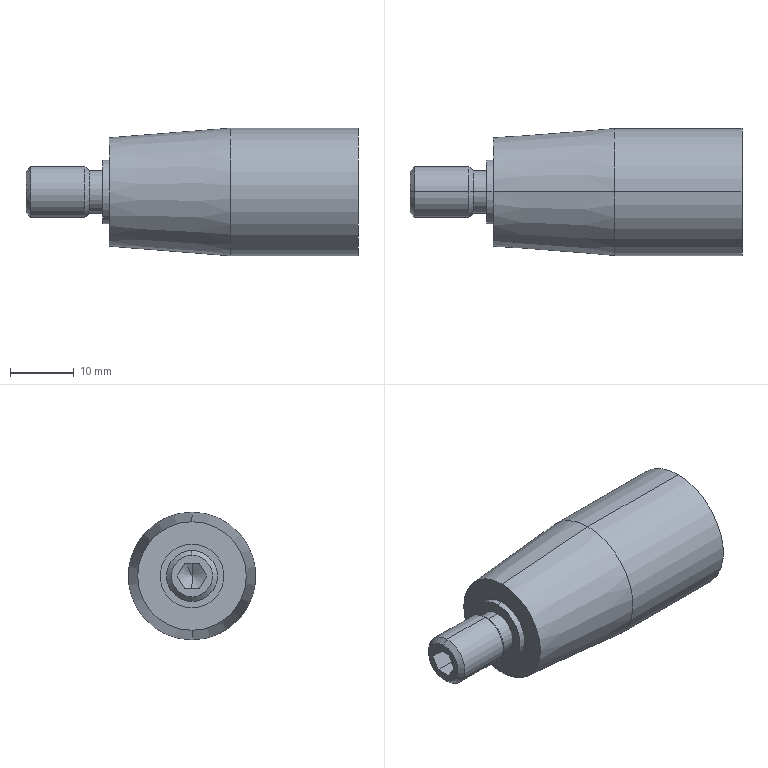Part | SolidWorks | features RefAxis 3, 3DProfileFeature 1, ICE 1, RevCut 1, Revolution 1 | 1 solid | 32 faces | box 52 x 20 x 20 mm | volume 11976 mm3 | plane 16 | cone 8 | cylinder 8 | commonest cylinder face diameters 6.647 x2 8 x2 10 x2 20 x2
STEP:
#1=CARTESIAN_POINT('',(-7.67,0.,0.));
#2=VERTEX_POINT('',#1);
#3=CARTESIAN_POINT('',(-9.,0.,2.309));
#4=VERTEX_POINT('',#3);
#5=CARTESIAN_POINT('',(-7.67,0.,0.));
#6=DIRECTION('',(-0.4991,0.,0.8666));
#7=VECTOR('',#6,1000.);
#8=LINE('',#5,#7);
#9=EDGE_CURVE('',#2,#4,#8,.T.);
#10=ORIENTED_EDGE('',*,*,#9,.F.);
#11=CARTESIAN_POINT('',(-9.,0.,-2.309));
#12=VERTEX_POINT('',#11);
#13=CARTESIAN_POINT('',(-7.67,0.,0.));
#14=DIRECTION('',(-0.4991,0.,-0.8666));
#15=VECTOR('',#14,1000.);
#16=LINE('',#13,#15);
#17=EDGE_CURVE('',#2,#12,#16,.T.);
#18=ORIENTED_EDGE('',*,*,#17,.T.);
#19=CARTESIAN_POINT('',(-9.,-1.155,-2.));
#20=VERTEX_POINT('',#19);
#21=CARTESIAN_POINT('',(-9.,0.,0.));
#22=DIRECTION('',(-1.,0.,0.));
#23=DIRECTION('',(0.,0.,1.));
#24=AXIS2_PLACEMENT_3D('',#21,#22,#23);
#25=CIRCLE('',#24,2.309);
#26=EDGE_CURVE('',#12,#20,#25,.T.);
#27=ORIENTED_EDGE('',*,*,#26,.T.);
#28=CARTESIAN_POINT('',(-9.,-2.309,0.));
#29=VERTEX_POINT('',#28);
#30=CARTESIAN_POINT('',(-9.,0.,0.));
#31=DIRECTION('',(-1.,0.,0.));
#32=DIRECTION('',(0.,0.,1.));
#33=AXIS2_PLACEMENT_3D('',#30,#31,#32);
#34=CIRCLE('',#33,2.309);
#35=EDGE_CURVE('',#20,#29,#34,.T.);
#36=ORIENTED_EDGE('',*,*,#35,.T.);
#37=CARTESIAN_POINT('',(-9.,-1.155,2.));
#38=VERTEX_POINT('',#37);
#39=CARTESIAN_POINT('',(-9.,0.,0.));
#40=DIRECTION('',(-1.,0.,0.));
#41=DIRECTION('',(0.,0.,1.));
#42=AXIS2_PLACEMENT_3D('',#39,#40,#41);
#43=CIRCLE('',#42,2.309);
#44=EDGE_CURVE('',#29,#38,#43,.T.);
#45=ORIENTED_EDGE('',*,*,#44,.T.);
#46=CARTESIAN_POINT('',(-9.,0.,0.));
#47=DIRECTION('',(-1.,0.,0.));
#48=DIRECTION('',(0.,0.,1.));
#49=AXIS2_PLACEMENT_3D('',#46,#47,#48);
#50=CIRCLE('',#49,2.309);
#51=EDGE_CURVE('',#38,#4,#50,.T.);
#52=ORIENTED_EDGE('',*,*,#51,.T.);
#53=EDGE_LOOP('',(#10,#18,#27,#36,#45,#52));
#54=FACE_OUTER_BOUND('',#53,.T.);
#55=CARTESIAN_POINT('',(-1007.67,0.,0.));
#56=DIRECTION('',(-1.,0.,0.));
#57=DIRECTION('',(0.,0.,1.));
#58=AXIS2_PLACEMENT_3D('',#55,#56,#57);
#59=CONICAL_SURFACE('',#58,1736.392,1.048);
#60=ADVANCED_FACE('',(#54),#59,.F.);
#61=CARTESIAN_POINT('',(39.,0.,10.));
#62=VERTEX_POINT('',#61);
#63=CARTESIAN_POINT('',(39.,0.,-10.));
#64=VERTEX_POINT('',#63);
#65=CARTESIAN_POINT('',(39.,0.,0.));
#66=DIRECTION('',(-1.,0.,0.));
#67=DIRECTION('',(0.,0.,1.));
#68=AXIS2_PLACEMENT_3D('',#65,#66,#67);
#69=CIRCLE('',#68,10.);
#70=EDGE_CURVE('',#62,#64,#69,.T.);
#71=ORIENTED_EDGE('',*,*,#70,.T.);
#72=CARTESIAN_POINT('',(19.,0.,-10.));
#73=VERTEX_POINT('',#72);
#74=CARTESIAN_POINT('',(39.,0.,-10.));
#75=DIRECTION('',(-1.,0.,0.));
#76=VECTOR('',#75,1000.);
#77=LINE('',#74,#76);
#78=EDGE_CURVE('',#64,#73,#77,.T.);
#79=ORIENTED_EDGE('',*,*,#78,.T.);
#80=CARTESIAN_POINT('',(19.,0.,10.));
#81=VERTEX_POINT('',#80);
#82=CARTESIAN_POINT('',(19.,0.,0.));
#83=DIRECTION('',(-1.,0.,0.));
#84=DIRECTION('',(0.,0.,1.));
#85=AXIS2_PLACEMENT_3D('',#82,#83,#84);
#86=CIRCLE('',#85,10.);
#87=EDGE_CURVE('',#81,#73,#86,.T.);
#88=ORIENTED_EDGE('',*,*,#87,.F.);
#89=CARTESIAN_POINT('',(39.,0.,10.));
#90=DIRECTION('',(-1.,0.,0.));
#91=VECTOR('',#90,1000.);
#92=LINE('',#89,#91);
#93=EDGE_CURVE('',#62,#81,#92,.T.);
#94=ORIENTED_EDGE('',*,*,#93,.F.);
#95=EDGE_LOOP('',(#71,#79,#88,#94));
#96=FACE_OUTER_BOUND('',#95,.T.);
#97=CARTESIAN_POINT('',(39.,0.,0.));
#98=DIRECTION('',(-1.,0.,0.));
#99=DIRECTION('',(0.,0.,1.));
#100=AXIS2_PLACEMENT_3D('',#97,#98,#99);
#101=CYLINDRICAL_SURFACE('',#100,10.);
#102=ADVANCED_FACE('',(#96),#101,.T.);
#103=CARTESIAN_POINT('',(0.,0.,8.5));
#104=VERTEX_POINT('',#103);
#105=CARTESIAN_POINT('',(0.,0.,-8.5));
#106=VERTEX_POINT('',#105);
#107=CARTESIAN_POINT('',(0.,0.,0.));
#108=DIRECTION('',(-1.,0.,0.));
#109=DIRECTION('',(0.,0.,1.));
#110=AXIS2_PLACEMENT_3D('',#107,#108,#109);
#111=CIRCLE('',#110,8.5);
#112=EDGE_CURVE('',#104,#106,#111,.T.);
#113=ORIENTED_EDGE('',*,*,#112,.F.);
#114=CARTESIAN_POINT('',(19.,0.,10.));
#115=DIRECTION('',(0.9969,0.,0.0787));
#116=VECTOR('',#115,1000.);
#117=LINE('',#114,#116);
#118=EDGE_CURVE('',#104,#81,#117,.T.);
#119=ORIENTED_EDGE('',*,*,#118,.T.);
#120=ORIENTED_EDGE('',*,*,#87,.T.);
#121=CARTESIAN_POINT('',(19.,0.,-10.));
#122=DIRECTION('',(0.9969,0.,-0.0787));
#123=VECTOR('',#122,1000.);
#124=LINE('',#121,#123);
#125=EDGE_CURVE('',#106,#73,#124,.T.);
#126=ORIENTED_EDGE('',*,*,#125,.F.);
#127=EDGE_LOOP('',(#113,#119,#120,#126));
#128=FACE_OUTER_BOUND('',#127,.T.);
#129=CARTESIAN_POINT('',(19.,0.,0.));
#130=DIRECTION('',(1.,0.,0.));
#131=DIRECTION('',(0.,0.,-1.));
#132=AXIS2_PLACEMENT_3D('',#129,#130,#131);
#133=CONICAL_SURFACE('',#132,10.,0.07878);
#134=ADVANCED_FACE('',(#128),#133,.T.);
#135=CARTESIAN_POINT('',(0.,0.,5.));
#136=VERTEX_POINT('',#135);
#137=CARTESIAN_POINT('',(0.,0.,-5.));
#138=VERTEX_POINT('',#137);
#139=CARTESIAN_POINT('',(0.,0.,0.));
#140=DIRECTION('',(-1.,0.,0.));
#141=DIRECTION('',(0.,0.,1.));
#142=AXIS2_PLACEMENT_3D('',#139,#140,#141);
#143=CIRCLE('',#142,5.);
#144=EDGE_CURVE('',#136,#138,#143,.T.);
#145=ORIENTED_EDGE('',*,*,#144,.T.);
#146=CARTESIAN_POINT('',(-1.,0.,-5.));
#147=VERTEX_POINT('',#146);
#148=CARTESIAN_POINT('',(39.,0.,-5.));
#149=DIRECTION('',(-1.,0.,0.));
#150=VECTOR('',#149,1000.);
#151=LINE('',#148,#150);
#152=EDGE_CURVE('',#138,#147,#151,.T.);
#153=ORIENTED_EDGE('',*,*,#152,.T.);
#154=CARTESIAN_POINT('',(-1.,0.,5.));
#155=VERTEX_POINT('',#154);
#156=CARTESIAN_POINT('',(-1.,0.,0.));
#157=DIRECTION('',(-1.,0.,0.));
#158=DIRECTION('',(0.,0.,1.));
#159=AXIS2_PLACEMENT_3D('',#156,#157,#158);
#160=CIRCLE('',#159,5.);
#161=EDGE_CURVE('',#155,#147,#160,.T.);
#162=ORIENTED_EDGE('',*,*,#161,.F.);
#163=CARTESIAN_POINT('',(39.,0.,5.));
#164=DIRECTION('',(-1.,0.,0.));
#165=VECTOR('',#164,1000.);
#166=LINE('',#163,#165);
#167=EDGE_CURVE('',#136,#155,#166,.T.);
#168=ORIENTED_EDGE('',*,*,#167,.F.);
#169=EDGE_LOOP('',(#145,#153,#162,#168));
#170=FACE_OUTER_BOUND('',#169,.T.);
#171=CARTESIAN_POINT('',(39.,0.,0.));
#172=DIRECTION('',(-1.,0.,0.));
#173=DIRECTION('',(0.,0.,1.));
#174=AXIS2_PLACEMENT_3D('',#171,#172,#173);
#175=CYLINDRICAL_SURFACE('',#174,5.);
#176=ADVANCED_FACE('',(#170),#175,.T.);
#177=CARTESIAN_POINT('',(-1.,0.,3.324));
#178=VERTEX_POINT('',#177);
#179=CARTESIAN_POINT('',(-1.,0.,-3.324));
#180=VERTEX_POINT('',#179);
#181=CARTESIAN_POINT('',(-1.,0.,0.));
#182=DIRECTION('',(-1.,0.,0.));
#183=DIRECTION('',(0.,0.,1.));
#184=AXIS2_PLACEMENT_3D('',#181,#182,#183);
#185=CIRCLE('',#184,3.324);
#186=EDGE_CURVE('',#178,#180,#185,.T.);
#187=ORIENTED_EDGE('',*,*,#186,.T.);
#188=CARTESIAN_POINT('',(-3.091,0.,-3.324));
#189=VERTEX_POINT('',#188);
#190=CARTESIAN_POINT('',(39.,0.,-3.324));
#191=DIRECTION('',(-1.,0.,0.));
#192=VECTOR('',#191,1000.);
#193=LINE('',#190,#192);
#194=EDGE_CURVE('',#180,#189,#193,.T.);
#195=ORIENTED_EDGE('',*,*,#194,.T.);
#196=CARTESIAN_POINT('',(-3.091,0.,3.324));
#197=VERTEX_POINT('',#196);
#198=CARTESIAN_POINT('',(-3.091,0.,0.));
#199=DIRECTION('',(-1.,0.,0.));
#200=DIRECTION('',(0.,0.,1.));
#201=AXIS2_PLACEMENT_3D('',#198,#199,#200);
#202=CIRCLE('',#201,3.324);
#203=EDGE_CURVE('',#197,#189,#202,.T.);
#204=ORIENTED_EDGE('',*,*,#203,.F.);
#205=CARTESIAN_POINT('',(39.,0.,3.324));
#206=DIRECTION('',(-1.,0.,0.));
#207=VECTOR('',#206,1000.);
#208=LINE('',#205,#207);
#209=EDGE_CURVE('',#178,#197,#208,.T.);
#210=ORIENTED_EDGE('',*,*,#209,.F.);
#211=EDGE_LOOP('',(#187,#195,#204,#210));
#212=FACE_OUTER_BOUND('',#211,.T.);
#213=CARTESIAN_POINT('',(39.,0.,0.));
#214=DIRECTION('',(-1.,0.,0.));
#215=DIRECTION('',(0.,0.,1.));
#216=AXIS2_PLACEMENT_3D('',#213,#214,#215);
#217=CYLINDRICAL_SURFACE('',#216,3.324);
#218=ADVANCED_FACE('',(#212),#217,.T.);
#219=ORIENTED_EDGE('',*,*,#203,.T.);
#220=CARTESIAN_POINT('',(-3.767,0.,-4.));
#221=VERTEX_POINT('',#220);
#222=CARTESIAN_POINT('',(-3.091,0.,-3.324));
#223=DIRECTION('',(-0.7071,0.,-0.7071));
#224=VECTOR('',#223,1000.);
#225=LINE('',#222,#224);
#226=EDGE_CURVE('',#189,#221,#225,.T.);
#227=ORIENTED_EDGE('',*,*,#226,.T.);
#228=CARTESIAN_POINT('',(-3.767,0.,4.));
#229=VERTEX_POINT('',#228);
#230=CARTESIAN_POINT('',(-3.767,0.,0.));
#231=DIRECTION('',(-1.,0.,0.));
#232=DIRECTION('',(0.,0.,1.));
#233=AXIS2_PLACEMENT_3D('',#230,#231,#232);
#234=CIRCLE('',#233,4.);
#235=EDGE_CURVE('',#229,#221,#234,.T.);
#236=ORIENTED_EDGE('',*,*,#235,.F.);
#237=CARTESIAN_POINT('',(-3.091,0.,3.324));
#238=DIRECTION('',(-0.7071,0.,0.7071));
#239=VECTOR('',#238,1000.);
#240=LINE('',#237,#239);
#241=EDGE_CURVE('',#197,#229,#240,.T.);
#242=ORIENTED_EDGE('',*,*,#241,.F.);
#243=EDGE_LOOP('',(#219,#227,#236,#242));
#244=FACE_OUTER_BOUND('',#243,.T.);
#245=CARTESIAN_POINT('',(-3.091,0.,0.));
#246=DIRECTION('',(-1.,0.,0.));
#247=DIRECTION('',(0.,0.,1.));
#248=AXIS2_PLACEMENT_3D('',#245,#246,#247);
#249=CONICAL_SURFACE('',#248,3.324,0.7854);
#250=ADVANCED_FACE('',(#244),#249,.T.);
#251=ORIENTED_EDGE('',*,*,#235,.T.);
#252=CARTESIAN_POINT('',(-12.233,0.,-4.));
#253=VERTEX_POINT('',#252);
#254=CARTESIAN_POINT('',(39.,0.,-4.));
#255=DIRECTION('',(-1.,0.,0.));
#256=VECTOR('',#255,1000.);
#257=LINE('',#254,#256);
#258=EDGE_CURVE('',#221,#253,#257,.T.);
#259=ORIENTED_EDGE('',*,*,#258,.T.);
#260=CARTESIAN_POINT('',(-12.233,0.,4.));
#261=VERTEX_POINT('',#260);
#262=CARTESIAN_POINT('',(-12.233,0.,0.));
#263=DIRECTION('',(-1.,0.,0.));
#264=DIRECTION('',(0.,0.,1.));
#265=AXIS2_PLACEMENT_3D('',#262,#263,#264);
#266=CIRCLE('',#265,4.);
#267=EDGE_CURVE('',#261,#253,#266,.T.);
#268=ORIENTED_EDGE('',*,*,#267,.F.);
#269=CARTESIAN_POINT('',(39.,0.,4.));
#270=DIRECTION('',(-1.,0.,0.));
#271=VECTOR('',#270,1000.);
#272=LINE('',#269,#271);
#273=EDGE_CURVE('',#229,#261,#272,.T.);
#274=ORIENTED_EDGE('',*,*,#273,.F.);
#275=EDGE_LOOP('',(#251,#259,#268,#274));
#276=FACE_OUTER_BOUND('',#275,.T.);
#277=CARTESIAN_POINT('',(39.,0.,0.));
#278=DIRECTION('',(-1.,0.,0.));
#279=DIRECTION('',(0.,0.,1.));
#280=AXIS2_PLACEMENT_3D('',#277,#278,#279);
#281=CYLINDRICAL_SURFACE('',#280,4.);
#282=ADVANCED_FACE('',(#276),#281,.T.);
#283=CARTESIAN_POINT('',(-13.,0.,3.233));
#284=VERTEX_POINT('',#283);
#285=CARTESIAN_POINT('',(-13.,0.,-3.233));
#286=VERTEX_POINT('',#285);
#287=CARTESIAN_POINT('',(-13.,0.,0.));
#288=DIRECTION('',(-1.,0.,0.));
#289=DIRECTION('',(0.,0.,1.));
#290=AXIS2_PLACEMENT_3D('',#287,#288,#289);
#291=CIRCLE('',#290,3.233);
#292=EDGE_CURVE('',#284,#286,#291,.T.);
#293=ORIENTED_EDGE('',*,*,#292,.F.);
#294=CARTESIAN_POINT('',(-12.233,0.,4.));
#295=DIRECTION('',(0.7071,0.,0.7071));
#296=VECTOR('',#295,1000.);
#297=LINE('',#294,#296);
#298=EDGE_CURVE('',#284,#261,#297,.T.);
#299=ORIENTED_EDGE('',*,*,#298,.T.);
#300=ORIENTED_EDGE('',*,*,#267,.T.);
#301=CARTESIAN_POINT('',(-12.233,0.,-4.));
#302=DIRECTION('',(0.7071,0.,-0.7071));
#303=VECTOR('',#302,1000.);
#304=LINE('',#301,#303);
#305=EDGE_CURVE('',#286,#253,#304,.T.);
#306=ORIENTED_EDGE('',*,*,#305,.F.);
#307=EDGE_LOOP('',(#293,#299,#300,#306));
#308=FACE_OUTER_BOUND('',#307,.T.);
#309=CARTESIAN_POINT('',(-12.233,0.,0.));
#310=DIRECTION('',(1.,0.,0.));
#311=DIRECTION('',(0.,0.,-1.));
#312=AXIS2_PLACEMENT_3D('',#309,#310,#311);
#313=CONICAL_SURFACE('',#312,4.,0.7854);
#314=ADVANCED_FACE('',(#308),#313,.T.);
#315=CARTESIAN_POINT('',(-13.,0.,0.));
#316=DIRECTION('',(-1.,0.,0.));
#317=DIRECTION('',(0.,0.,1.));
#318=AXIS2_PLACEMENT_3D('',#315,#316,#317);
#319=CIRCLE('',#318,3.233);
#320=EDGE_CURVE('',#286,#284,#319,.T.);
#321=ORIENTED_EDGE('',*,*,#320,.T.);
#322=ORIENTED_EDGE('',*,*,#292,.T.);
#323=EDGE_LOOP('',(#321,#322));
#324=FACE_OUTER_BOUND('',#323,.T.);
#325=CARTESIAN_POINT('',(-13.,2.309,0.));
#326=VERTEX_POINT('',#325);
#327=CARTESIAN_POINT('',(-13.,1.155,2.));
#328=VERTEX_POINT('',#327);
#329=CARTESIAN_POINT('',(-13.,2.309,0.));
#330=DIRECTION('',(0.,-0.5,0.866));
#331=VECTOR('',#330,1000.);
#332=LINE('',#329,#331);
#333=EDGE_CURVE('',#326,#328,#332,.T.);
#334=ORIENTED_EDGE('',*,*,#333,.T.);
#335=CARTESIAN_POINT('',(-13.,-1.155,2.));
#336=VERTEX_POINT('',#335);
#337=CARTESIAN_POINT('',(-13.,1.155,2.));
#338=DIRECTION('',(0.,-1.,0.));
#339=VECTOR('',#338,1000.);
#340=LINE('',#337,#339);
#341=EDGE_CURVE('',#328,#336,#340,.T.);
#342=ORIENTED_EDGE('',*,*,#341,.T.);
#343=CARTESIAN_POINT('',(-13.,-2.309,0.));
#344=VERTEX_POINT('',#343);
#345=CARTESIAN_POINT('',(-13.,-1.155,2.));
#346=DIRECTION('',(0.,-0.5,-0.866));
#347=VECTOR('',#346,1000.);
#348=LINE('',#345,#347);
#349=EDGE_CURVE('',#336,#344,#348,.T.);
#350=ORIENTED_EDGE('',*,*,#349,.T.);
#351=CARTESIAN_POINT('',(-13.,-1.155,-2.));
#352=VERTEX_POINT('',#351);
#353=CARTESIAN_POINT('',(-13.,-2.309,0.));
#354=DIRECTION('',(0.,0.5,-0.866));
#355=VECTOR('',#354,1000.);
#356=LINE('',#353,#355);
#357=EDGE_CURVE('',#344,#352,#356,.T.);
#358=ORIENTED_EDGE('',*,*,#357,.T.);
#359=CARTESIAN_POINT('',(-13.,1.155,-2.));
#360=VERTEX_POINT('',#359);
#361=CARTESIAN_POINT('',(-13.,-1.155,-2.));
#362=DIRECTION('',(0.,1.,0.));
#363=VECTOR('',#362,1000.);
#364=LINE('',#361,#363);
#365=EDGE_CURVE('',#352,#360,#364,.T.);
#366=ORIENTED_EDGE('',*,*,#365,.T.);
#367=CARTESIAN_POINT('',(-13.,1.155,-2.));
#368=DIRECTION('',(0.,0.5,0.866));
#369=VECTOR('',#368,1000.);
#370=LINE('',#367,#369);
#371=EDGE_CURVE('',#360,#326,#370,.T.);
#372=ORIENTED_EDGE('',*,*,#371,.T.);
#373=EDGE_LOOP('',(#334,#342,#350,#358,#366,#372));
#374=FACE_BOUND('',#373,.T.);
#375=CARTESIAN_POINT('',(-13.,0.,0.));
#376=DIRECTION('',(1.,0.,0.));
#377=DIRECTION('',(0.,0.,-1.));
#378=AXIS2_PLACEMENT_3D('',#375,#376,#377);
#379=PLANE('',#378);
#380=ADVANCED_FACE('',(#324,#374),#379,.F.);
#381=ORIENTED_EDGE('',*,*,#298,.F.);
#382=ORIENTED_EDGE('',*,*,#320,.F.);
#383=ORIENTED_EDGE('',*,*,#305,.T.);
#384=CARTESIAN_POINT('',(-12.233,0.,0.));
#385=DIRECTION('',(-1.,0.,0.));
#386=DIRECTION('',(0.,0.,1.));
#387=AXIS2_PLACEMENT_3D('',#384,#385,#386);
#388=CIRCLE('',#387,4.);
#389=EDGE_CURVE('',#253,#261,#388,.T.);
#390=ORIENTED_EDGE('',*,*,#389,.T.);
#391=EDGE_LOOP('',(#381,#382,#383,#390));
#392=FACE_OUTER_BOUND('',#391,.T.);
#393=CARTESIAN_POINT('',(-12.233,0.,0.));
#394=DIRECTION('',(1.,0.,0.));
#395=DIRECTION('',(0.,0.,-1.));
#396=AXIS2_PLACEMENT_3D('',#393,#394,#395);
#397=CONICAL_SURFACE('',#396,4.,0.7854);
#398=ADVANCED_FACE('',(#392),#397,.T.);
#399=ORIENTED_EDGE('',*,*,#258,.F.);
#400=CARTESIAN_POINT('',(-3.767,0.,0.));
#401=DIRECTION('',(-1.,0.,0.));
#402=DIRECTION('',(0.,0.,1.));
#403=AXIS2_PLACEMENT_3D('',#400,#401,#402);
#404=CIRCLE('',#403,4.);
#405=EDGE_CURVE('',#221,#229,#404,.T.);
#406=ORIENTED_EDGE('',*,*,#405,.T.);
#407=ORIENTED_EDGE('',*,*,#273,.T.);
#408=ORIENTED_EDGE('',*,*,#389,.F.);
#409=EDGE_LOOP('',(#399,#406,#407,#408));
#410=FACE_OUTER_BOUND('',#409,.T.);
#411=CARTESIAN_POINT('',(39.,0.,0.));
#412=DIRECTION('',(-1.,0.,0.));
#413=DIRECTION('',(0.,0.,1.));
#414=AXIS2_PLACEMENT_3D('',#411,#412,#413);
#415=CYLINDRICAL_SURFACE('',#414,4.);
#416=ADVANCED_FACE('',(#410),#415,.T.);
#417=ORIENTED_EDGE('',*,*,#226,.F.);
#418=CARTESIAN_POINT('',(-3.091,0.,0.));
#419=DIRECTION('',(-1.,0.,0.));
#420=DIRECTION('',(0.,0.,1.));
#421=AXIS2_PLACEMENT_3D('',#418,#419,#420);
#422=CIRCLE('',#421,3.324);
#423=EDGE_CURVE('',#189,#197,#422,.T.);
#424=ORIENTED_EDGE('',*,*,#423,.T.);
#425=ORIENTED_EDGE('',*,*,#241,.T.);
#426=ORIENTED_EDGE('',*,*,#405,.F.);
#427=EDGE_LOOP('',(#417,#424,#425,#426));
#428=FACE_OUTER_BOUND('',#427,.T.);
#429=CARTESIAN_POINT('',(-3.091,0.,0.));
#430=DIRECTION('',(-1.,0.,0.));
#431=DIRECTION('',(0.,0.,1.));
#432=AXIS2_PLACEMENT_3D('',#429,#430,#431);
#433=CONICAL_SURFACE('',#432,3.324,0.7854);
#434=ADVANCED_FACE('',(#428),#433,.T.);
#435=ORIENTED_EDGE('',*,*,#194,.F.);
#436=CARTESIAN_POINT('',(-1.,0.,0.));
#437=DIRECTION('',(-1.,0.,0.));
#438=DIRECTION('',(0.,0.,1.));
#439=AXIS2_PLACEMENT_3D('',#436,#437,#438);
#440=CIRCLE('',#439,3.324);
#441=EDGE_CURVE('',#180,#178,#440,.T.);
#442=ORIENTED_EDGE('',*,*,#441,.T.);
#443=ORIENTED_EDGE('',*,*,#209,.T.);
#444=ORIENTED_EDGE('',*,*,#423,.F.);
#445=EDGE_LOOP('',(#435,#442,#443,#444));
#446=FACE_OUTER_BOUND('',#445,.T.);
#447=CARTESIAN_POINT('',(39.,0.,0.));
#448=DIRECTION('',(-1.,0.,0.));
#449=DIRECTION('',(0.,0.,1.));
#450=AXIS2_PLACEMENT_3D('',#447,#448,#449);
#451=CYLINDRICAL_SURFACE('',#450,3.324);
#452=ADVANCED_FACE('',(#446),#451,.T.);
#453=ORIENTED_EDGE('',*,*,#186,.F.);
#454=ORIENTED_EDGE('',*,*,#441,.F.);
#455=EDGE_LOOP('',(#453,#454));
#456=FACE_BOUND('',#455,.T.);
#457=ORIENTED_EDGE('',*,*,#161,.T.);
#458=CARTESIAN_POINT('',(-1.,0.,0.));
#459=DIRECTION('',(-1.,0.,0.));
#460=DIRECTION('',(0.,0.,1.));
#461=AXIS2_PLACEMENT_3D('',#458,#459,#460);
#462=CIRCLE('',#461,5.);
#463=EDGE_CURVE('',#147,#155,#462,.T.);
#464=ORIENTED_EDGE('',*,*,#463,.T.);
#465=EDGE_LOOP('',(#457,#464));
#466=FACE_OUTER_BOUND('',#465,.T.);
#467=CARTESIAN_POINT('',(-1.,3.324,0.));
#468=DIRECTION('',(1.,0.,0.));
#469=DIRECTION('',(0.,0.,-1.));
#470=AXIS2_PLACEMENT_3D('',#467,#468,#469);
#471=PLANE('',#470);
#472=ADVANCED_FACE('',(#456,#466),#471,.F.);
#473=ORIENTED_EDGE('',*,*,#152,.F.);
#474=CARTESIAN_POINT('',(0.,0.,0.));
#475=DIRECTION('',(-1.,0.,0.));
#476=DIRECTION('',(0.,0.,1.));
#477=AXIS2_PLACEMENT_3D('',#474,#475,#476);
#478=CIRCLE('',#477,5.);
#479=EDGE_CURVE('',#138,#136,#478,.T.);
#480=ORIENTED_EDGE('',*,*,#479,.T.);
#481=ORIENTED_EDGE('',*,*,#167,.T.);
#482=ORIENTED_EDGE('',*,*,#463,.F.);
#483=EDGE_LOOP('',(#473,#480,#481,#482));
#484=FACE_OUTER_BOUND('',#483,.T.);
#485=CARTESIAN_POINT('',(39.,0.,0.));
#486=DIRECTION('',(-1.,0.,0.));
#487=DIRECTION('',(0.,0.,1.));
#488=AXIS2_PLACEMENT_3D('',#485,#486,#487);
#489=CYLINDRICAL_SURFACE('',#488,5.);
#490=ADVANCED_FACE('',(#484),#489,.T.);
#491=ORIENTED_EDGE('',*,*,#144,.F.);
#492=ORIENTED_EDGE('',*,*,#479,.F.);
#493=EDGE_LOOP('',(#491,#492));
#494=FACE_BOUND('',#493,.T.);
#495=CARTESIAN_POINT('',(0.,0.,0.));
#496=DIRECTION('',(-1.,0.,0.));
#497=DIRECTION('',(0.,0.,1.));
#498=AXIS2_PLACEMENT_3D('',#495,#496,#497);
#499=CIRCLE('',#498,8.5);
#500=EDGE_CURVE('',#106,#104,#499,.T.);
#501=ORIENTED_EDGE('',*,*,#500,.T.);
#502=ORIENTED_EDGE('',*,*,#112,.T.);
#503=EDGE_LOOP('',(#501,#502));
#504=FACE_OUTER_BOUND('',#503,.T.);
#505=CARTESIAN_POINT('',(0.,5.,0.));
#506=DIRECTION('',(1.,0.,0.));
#507=DIRECTION('',(0.,0.,-1.));
#508=AXIS2_PLACEMENT_3D('',#505,#506,#507);
#509=PLANE('',#508);
#510=ADVANCED_FACE('',(#494,#504),#509,.F.);
#511=ORIENTED_EDGE('',*,*,#118,.F.);
#512=ORIENTED_EDGE('',*,*,#500,.F.);
#513=ORIENTED_EDGE('',*,*,#125,.T.);
#514=CARTESIAN_POINT('',(19.,0.,0.));
#515=DIRECTION('',(-1.,0.,0.));
#516=DIRECTION('',(0.,0.,1.));
#517=AXIS2_PLACEMENT_3D('',#514,#515,#516);
#518=CIRCLE('',#517,10.);
#519=EDGE_CURVE('',#73,#81,#518,.T.);
#520=ORIENTED_EDGE('',*,*,#519,.T.);
#521=EDGE_LOOP('',(#511,#512,#513,#520));
#522=FACE_OUTER_BOUND('',#521,.T.);
#523=CARTESIAN_POINT('',(19.,0.,0.));
#524=DIRECTION('',(1.,0.,0.));
#525=DIRECTION('',(0.,0.,-1.));
#526=AXIS2_PLACEMENT_3D('',#523,#524,#525);
#527=CONICAL_SURFACE('',#526,10.,0.07878);
#528=ADVANCED_FACE('',(#522),#527,.T.);
#529=ORIENTED_EDGE('',*,*,#78,.F.);
#530=CARTESIAN_POINT('',(39.,0.,0.));
#531=DIRECTION('',(-1.,0.,0.));
#532=DIRECTION('',(0.,0.,1.));
#533=AXIS2_PLACEMENT_3D('',#530,#531,#532);
#534=CIRCLE('',#533,10.);
#535=EDGE_CURVE('',#64,#62,#534,.T.);
#536=ORIENTED_EDGE('',*,*,#535,.T.);
#537=ORIENTED_EDGE('',*,*,#93,.T.);
#538=ORIENTED_EDGE('',*,*,#519,.F.);
#539=EDGE_LOOP('',(#529,#536,#537,#538));
#540=FACE_OUTER_BOUND('',#539,.T.);
#541=CARTESIAN_POINT('',(39.,0.,0.));
#542=DIRECTION('',(-1.,0.,0.));
#543=DIRECTION('',(0.,0.,1.));
#544=AXIS2_PLACEMENT_3D('',#541,#542,#543);
#545=CYLINDRICAL_SURFACE('',#544,10.);
#546=ADVANCED_FACE('',(#540),#545,.T.);
#547=ORIENTED_EDGE('',*,*,#70,.F.);
#548=ORIENTED_EDGE('',*,*,#535,.F.);
#549=EDGE_LOOP('',(#547,#548));
#550=FACE_OUTER_BOUND('',#549,.T.);
#551=CARTESIAN_POINT('',(39.,10.,0.));
#552=DIRECTION('',(-1.,0.,0.));
#553=DIRECTION('',(0.,0.,1.));
#554=AXIS2_PLACEMENT_3D('',#551,#552,#553);
#555=PLANE('',#554);
#556=ADVANCED_FACE('',(#550),#555,.F.);
#557=ORIENTED_EDGE('',*,*,#333,.F.);
#558=CARTESIAN_POINT('',(-9.,2.309,0.));
#559=VERTEX_POINT('',#558);
#560=CARTESIAN_POINT('',(-9.,2.309,0.));
#561=DIRECTION('',(-1.,0.,0.));
#562=VECTOR('',#561,1000.);
#563=LINE('',#560,#562);
#564=EDGE_CURVE('',#559,#326,#563,.T.);
#565=ORIENTED_EDGE('',*,*,#564,.F.);
#566=CARTESIAN_POINT('',(-9.,1.155,2.));
#567=VERTEX_POINT('',#566);
#568=CARTESIAN_POINT('',(-9.,2.309,0.));
#569=DIRECTION('',(0.,-0.5,0.866));
#570=VECTOR('',#569,1000.);
#571=LINE('',#568,#570);
#572=EDGE_CURVE('',#559,#567,#571,.T.);
#573=ORIENTED_EDGE('',*,*,#572,.T.);
#574=CARTESIAN_POINT('',(-9.,1.155,2.));
#575=DIRECTION('',(-1.,0.,0.));
#576=VECTOR('',#575,1000.);
#577=LINE('',#574,#576);
#578=EDGE_CURVE('',#567,#328,#577,.T.);
#579=ORIENTED_EDGE('',*,*,#578,.T.);
#580=EDGE_LOOP('',(#557,#565,#573,#579));
#581=FACE_OUTER_BOUND('',#580,.T.);
#582=CARTESIAN_POINT('',(-9.,2.309,0.));
#583=DIRECTION('',(0.,-0.866,-0.5));
#584=DIRECTION('',(0.,0.5,-0.866));
#585=AXIS2_PLACEMENT_3D('',#582,#583,#584);
#586=PLANE('',#585);
#587=ADVANCED_FACE('',(#581),#586,.T.);
#588=ORIENTED_EDGE('',*,*,#341,.F.);
#589=ORIENTED_EDGE('',*,*,#578,.F.);
#590=CARTESIAN_POINT('',(-9.,1.155,2.));
#591=DIRECTION('',(0.,-1.,0.));
#592=VECTOR('',#591,1000.);
#593=LINE('',#590,#592);
#594=EDGE_CURVE('',#567,#38,#593,.T.);
#595=ORIENTED_EDGE('',*,*,#594,.T.);
#596=CARTESIAN_POINT('',(-9.,-1.155,2.));
#597=DIRECTION('',(-1.,0.,0.));
#598=VECTOR('',#597,1000.);
#599=LINE('',#596,#598);
#600=EDGE_CURVE('',#38,#336,#599,.T.);
#601=ORIENTED_EDGE('',*,*,#600,.T.);
#602=EDGE_LOOP('',(#588,#589,#595,#601));
#603=FACE_OUTER_BOUND('',#602,.T.);
#604=CARTESIAN_POINT('',(-9.,1.155,2.));
#605=DIRECTION('',(0.,0.,-1.));
#606=DIRECTION('',(-1.,0.,0.));
#607=AXIS2_PLACEMENT_3D('',#604,#605,#606);
#608=PLANE('',#607);
#609=ADVANCED_FACE('',(#603),#608,.T.);
#610=ORIENTED_EDGE('',*,*,#349,.F.);
#611=ORIENTED_EDGE('',*,*,#600,.F.);
#612=CARTESIAN_POINT('',(-9.,-1.155,2.));
#613=DIRECTION('',(0.,-0.5,-0.866));
#614=VECTOR('',#613,1000.);
#615=LINE('',#612,#614);
#616=EDGE_CURVE('',#38,#29,#615,.T.);
#617=ORIENTED_EDGE('',*,*,#616,.T.);
#618=CARTESIAN_POINT('',(-9.,-2.309,0.));
#619=DIRECTION('',(-1.,0.,0.));
#620=VECTOR('',#619,1000.);
#621=LINE('',#618,#620);
#622=EDGE_CURVE('',#29,#344,#621,.T.);
#623=ORIENTED_EDGE('',*,*,#622,.T.);
#624=EDGE_LOOP('',(#610,#611,#617,#623));
#625=FACE_OUTER_BOUND('',#624,.T.);
#626=CARTESIAN_POINT('',(-9.,-1.155,2.));
#627=DIRECTION('',(0.,0.866,-0.5));
#628=DIRECTION('',(0.,0.5,0.866));
#629=AXIS2_PLACEMENT_3D('',#626,#627,#628);
#630=PLANE('',#629);
#631=ADVANCED_FACE('',(#625),#630,.T.);
#632=ORIENTED_EDGE('',*,*,#357,.F.);
#633=ORIENTED_EDGE('',*,*,#622,.F.);
#634=CARTESIAN_POINT('',(-9.,-2.309,0.));
#635=DIRECTION('',(0.,0.5,-0.866));
#636=VECTOR('',#635,1000.);
#637=LINE('',#634,#636);
#638=EDGE_CURVE('',#29,#20,#637,.T.);
#639=ORIENTED_EDGE('',*,*,#638,.T.);
#640=CARTESIAN_POINT('',(-9.,-1.155,-2.));
#641=DIRECTION('',(-1.,0.,0.));
#642=VECTOR('',#641,1000.);
#643=LINE('',#640,#642);
#644=EDGE_CURVE('',#20,#352,#643,.T.);
#645=ORIENTED_EDGE('',*,*,#644,.T.);
#646=EDGE_LOOP('',(#632,#633,#639,#645));
#647=FACE_OUTER_BOUND('',#646,.T.);
#648=CARTESIAN_POINT('',(-9.,-2.309,0.));
#649=DIRECTION('',(0.,0.866,0.5));
#650=DIRECTION('',(0.,-0.5,0.866));
#651=AXIS2_PLACEMENT_3D('',#648,#649,#650);
#652=PLANE('',#651);
#653=ADVANCED_FACE('',(#647),#652,.T.);
#654=ORIENTED_EDGE('',*,*,#365,.F.);
#655=ORIENTED_EDGE('',*,*,#644,.F.);
#656=CARTESIAN_POINT('',(-9.,1.155,-2.));
#657=VERTEX_POINT('',#656);
#658=CARTESIAN_POINT('',(-9.,-1.155,-2.));
#659=DIRECTION('',(0.,1.,0.));
#660=VECTOR('',#659,1000.);
#661=LINE('',#658,#660);
#662=EDGE_CURVE('',#20,#657,#661,.T.);
#663=ORIENTED_EDGE('',*,*,#662,.T.);
#664=CARTESIAN_POINT('',(-9.,1.155,-2.));
#665=DIRECTION('',(-1.,0.,0.));
#666=VECTOR('',#665,1000.);
#667=LINE('',#664,#666);
#668=EDGE_CURVE('',#657,#360,#667,.T.);
#669=ORIENTED_EDGE('',*,*,#668,.T.);
#670=EDGE_LOOP('',(#654,#655,#663,#669));
#671=FACE_OUTER_BOUND('',#670,.T.);
#672=CARTESIAN_POINT('',(-9.,-1.155,-2.));
#673=DIRECTION('',(0.,0.,1.));
#674=DIRECTION('',(1.,0.,0.));
#675=AXIS2_PLACEMENT_3D('',#672,#673,#674);
#676=PLANE('',#675);
#677=ADVANCED_FACE('',(#671),#676,.T.);
#678=ORIENTED_EDGE('',*,*,#371,.F.);
#679=ORIENTED_EDGE('',*,*,#668,.F.);
#680=CARTESIAN_POINT('',(-9.,1.155,-2.));
#681=DIRECTION('',(0.,0.5,0.866));
#682=VECTOR('',#681,1000.);
#683=LINE('',#680,#682);
#684=EDGE_CURVE('',#657,#559,#683,.T.);
#685=ORIENTED_EDGE('',*,*,#684,.T.);
#686=ORIENTED_EDGE('',*,*,#564,.T.);
#687=EDGE_LOOP('',(#678,#679,#685,#686));
#688=FACE_OUTER_BOUND('',#687,.T.);
#689=CARTESIAN_POINT('',(-9.,1.155,-2.));
#690=DIRECTION('',(0.,-0.866,0.5));
#691=DIRECTION('',(0.,-0.5,-0.866));
#692=AXIS2_PLACEMENT_3D('',#689,#690,#691);
#693=PLANE('',#692);
#694=ADVANCED_FACE('',(#688),#693,.T.);
#695=CARTESIAN_POINT('',(-9.,0.,0.));
#696=DIRECTION('',(-1.,0.,0.));
#697=DIRECTION('',(0.,0.,1.));
#698=AXIS2_PLACEMENT_3D('',#695,#696,#697);
#699=CIRCLE('',#698,2.309);
#700=EDGE_CURVE('',#567,#559,#699,.T.);
#701=ORIENTED_EDGE('',*,*,#700,.F.);
#702=ORIENTED_EDGE('',*,*,#572,.F.);
#703=EDGE_LOOP('',(#701,#702));
#704=FACE_OUTER_BOUND('',#703,.T.);
#705=CARTESIAN_POINT('',(-9.,0.,0.));
#706=DIRECTION('',(1.,0.,0.));
#707=DIRECTION('',(0.,0.,-1.));
#708=AXIS2_PLACEMENT_3D('',#705,#706,#707);
#709=PLANE('',#708);
#710=ADVANCED_FACE('',(#704),#709,.T.);
#711=CARTESIAN_POINT('',(-9.,0.,0.));
#712=DIRECTION('',(-1.,0.,0.));
#713=DIRECTION('',(0.,0.,1.));
#714=AXIS2_PLACEMENT_3D('',#711,#712,#713);
#715=CIRCLE('',#714,2.309);
#716=EDGE_CURVE('',#559,#657,#715,.T.);
#717=ORIENTED_EDGE('',*,*,#716,.F.);
#718=ORIENTED_EDGE('',*,*,#684,.F.);
#719=EDGE_LOOP('',(#717,#718));
#720=FACE_OUTER_BOUND('',#719,.T.);
#721=CARTESIAN_POINT('',(-9.,0.,0.));
#722=DIRECTION('',(1.,0.,0.));
#723=DIRECTION('',(0.,0.,-1.));
#724=AXIS2_PLACEMENT_3D('',#721,#722,#723);
#725=PLANE('',#724);
#726=ADVANCED_FACE('',(#720),#725,.T.);
#727=CARTESIAN_POINT('',(-9.,0.,0.));
#728=DIRECTION('',(-1.,0.,0.));
#729=DIRECTION('',(0.,0.,1.));
#730=AXIS2_PLACEMENT_3D('',#727,#728,#729);
#731=CIRCLE('',#730,2.309);
#732=EDGE_CURVE('',#657,#12,#731,.T.);
#733=ORIENTED_EDGE('',*,*,#732,.F.);
#734=ORIENTED_EDGE('',*,*,#662,.F.);
#735=ORIENTED_EDGE('',*,*,#26,.F.);
#736=EDGE_LOOP('',(#733,#734,#735));
#737=FACE_OUTER_BOUND('',#736,.T.);
#738=CARTESIAN_POINT('',(-9.,0.,0.));
#739=DIRECTION('',(1.,0.,0.));
#740=DIRECTION('',(0.,0.,-1.));
#741=AXIS2_PLACEMENT_3D('',#738,#739,#740);
#742=PLANE('',#741);
#743=ADVANCED_FACE('',(#737),#742,.T.);
#744=ORIENTED_EDGE('',*,*,#35,.F.);
#745=ORIENTED_EDGE('',*,*,#638,.F.);
#746=EDGE_LOOP('',(#744,#745));
#747=FACE_OUTER_BOUND('',#746,.T.);
#748=CARTESIAN_POINT('',(-9.,0.,0.));
#749=DIRECTION('',(1.,0.,0.));
#750=DIRECTION('',(0.,0.,-1.));
#751=AXIS2_PLACEMENT_3D('',#748,#749,#750);
#752=PLANE('',#751);
#753=ADVANCED_FACE('',(#747),#752,.T.);
#754=ORIENTED_EDGE('',*,*,#44,.F.);
#755=ORIENTED_EDGE('',*,*,#616,.F.);
#756=EDGE_LOOP('',(#754,#755));
#757=FACE_OUTER_BOUND('',#756,.T.);
#758=CARTESIAN_POINT('',(-9.,0.,0.));
#759=DIRECTION('',(1.,0.,0.));
#760=DIRECTION('',(0.,0.,-1.));
#761=AXIS2_PLACEMENT_3D('',#758,#759,#760);
#762=PLANE('',#761);
#763=ADVANCED_FACE('',(#757),#762,.T.);
#764=ORIENTED_EDGE('',*,*,#51,.F.);
#765=ORIENTED_EDGE('',*,*,#594,.F.);
#766=CARTESIAN_POINT('',(-9.,0.,0.));
#767=DIRECTION('',(-1.,0.,0.));
#768=DIRECTION('',(0.,0.,1.));
#769=AXIS2_PLACEMENT_3D('',#766,#767,#768);
#770=CIRCLE('',#769,2.309);
#771=EDGE_CURVE('',#4,#567,#770,.T.);
#772=ORIENTED_EDGE('',*,*,#771,.F.);
#773=EDGE_LOOP('',(#764,#765,#772));
#774=FACE_OUTER_BOUND('',#773,.T.);
#775=CARTESIAN_POINT('',(-9.,0.,0.));
#776=DIRECTION('',(1.,0.,0.));
#777=DIRECTION('',(0.,0.,-1.));
#778=AXIS2_PLACEMENT_3D('',#775,#776,#777);
#779=PLANE('',#778);
#780=ADVANCED_FACE('',(#774),#779,.T.);
#781=ORIENTED_EDGE('',*,*,#17,.F.);
#782=ORIENTED_EDGE('',*,*,#9,.T.);
#783=ORIENTED_EDGE('',*,*,#771,.T.);
#784=ORIENTED_EDGE('',*,*,#700,.T.);
#785=ORIENTED_EDGE('',*,*,#716,.T.);
#786=ORIENTED_EDGE('',*,*,#732,.T.);
#787=EDGE_LOOP('',(#781,#782,#783,#784,#785,#786));
#788=FACE_OUTER_BOUND('',#787,.T.);
#789=CARTESIAN_POINT('',(-1007.67,0.,0.));
#790=DIRECTION('',(-1.,0.,0.));
#791=DIRECTION('',(0.,0.,1.));
#792=AXIS2_PLACEMENT_3D('',#789,#790,#791);
#793=CONICAL_SURFACE('',#792,1736.392,1.048);
#794=ADVANCED_FACE('',(#788),#793,.F.);
#795=CLOSED_SHELL('',(#60,#102,#134,#176,#218,#250,#282,#314,#380,#398,#416,#434,#452,#472,#490,#510,#528,#546,#556,#587,#609,#631,#653,#677,#694,#710,#726,#743,#753,#763,#780,#794));
#796=MANIFOLD_SOLID_BREP('',#795);
#797=CARTESIAN_POINT('',(0.,0.,0.));
#798=DIRECTION('',(0.,0.,1.));
#799=DIRECTION('',(1.,0.,0.));
#800=AXIS2_PLACEMENT_3D('',#797,#798,#799);
#801=(LENGTH_UNIT()NAMED_UNIT(*)SI_UNIT(.MILLI.,.METRE.));
#802=UNCERTAINTY_MEASURE_WITH_UNIT(LENGTH_MEASURE(0.00001),#801,'','');
#803=(NAMED_UNIT(*)PLANE_ANGLE_UNIT()SI_UNIT($,.RADIAN.));
#804=(NAMED_UNIT(*)SI_UNIT($,.STERADIAN.)SOLID_ANGLE_UNIT());
#805=(GEOMETRIC_REPRESENTATION_CONTEXT(3)GLOBAL_UNCERTAINTY_ASSIGNED_CONTEXT((#802))GLOBAL_UNIT_ASSIGNED_CONTEXT((#801,#803,#804))REPRESENTATION_CONTEXT('',''));
#806=ADVANCED_BREP_SHAPE_REPRESENTATION('',(#796,#800),#805);